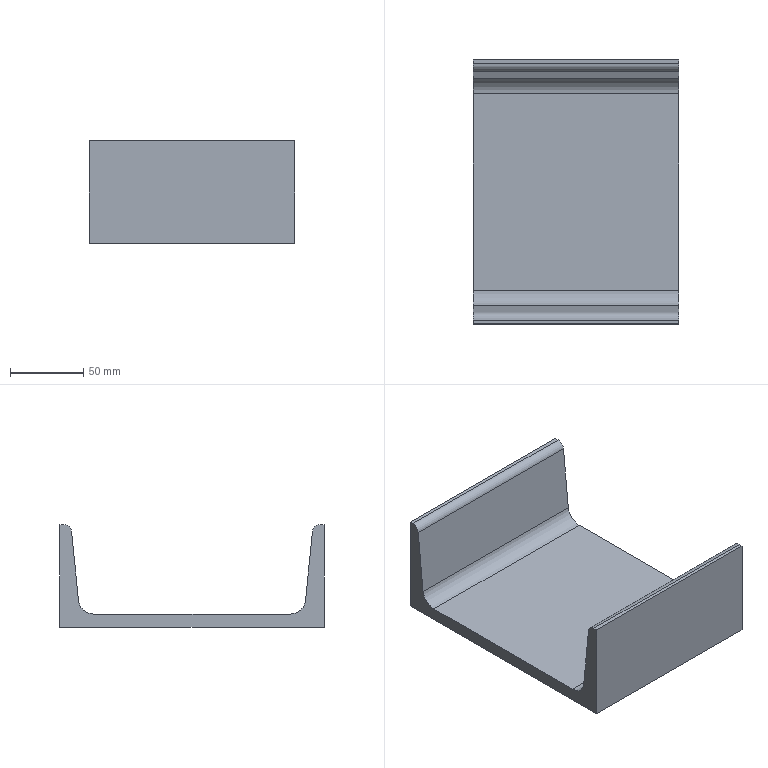Part | STEP file | 18# B Channel 140 (GB_INTERCHANGEABLE_PARTS_TM_SS 18X140)_GB_INTERCHANGEABLE_PARTS_TM_SS 18X140 | 1 solid | 14 faces | box 140 x 180 x 70 mm | volume 410063 mm3 | plane 10 | cylinder 4 | commonest cylinder face diameters 10.5 x2 21 x2
STEP:
#1=CARTESIAN_POINT('',(0.,0.,0.));
#2=DIRECTION('',(0.,0.,1.));
#3=DIRECTION('',(1.,0.,0.));
#4=AXIS2_PLACEMENT_3D('',#1,#2,#3);
#5=CARTESIAN_POINT('',(140.,82.077,65.272));
#6=VERTEX_POINT('',#5);
#7=CARTESIAN_POINT('',(140.,77.396,18.455));
#8=VERTEX_POINT('',#7);
#9=CARTESIAN_POINT('',(140.,76.45,9.));
#10=DIRECTION('',(0.,-0.0995,-0.995));
#11=VECTOR('',#10,1.);
#12=LINE('',#9,#11);
#13=CARTESIAN_POINT('',(140.,76.45,9.));
#14=DIRECTION('',(0.,0.995,-0.0995));
#15=DIRECTION('',(0.,0.0995,0.995));
#16=AXIS2_PLACEMENT_3D('',#13,#14,#15);
#17=PLANE('',#16);
#18=CARTESIAN_POINT('',(0.,0.));
#19=DIRECTION('',(-1.,0.));
#20=VECTOR('',#19,1.);
#21=LINE('',#18,#20);
#22=(GEOMETRIC_REPRESENTATION_CONTEXT(2)PARAMETRIC_REPRESENTATION_CONTEXT()REPRESENTATION_CONTEXT('',''));
#23=DEFINITIONAL_REPRESENTATION('',(#21),#22);
#24=PCURVE('',#17,#23);
#25=CARTESIAN_POINT('',(140.,75.55,0.));
#26=DIRECTION('',(1.,0.,0.));
#27=DIRECTION('',(0.,0.,-1.));
#28=AXIS2_PLACEMENT_3D('',#25,#26,#27);
#29=PLANE('',#28);
#30=CARTESIAN_POINT('',(-9.,0.9));
#31=DIRECTION('',(0.995,-0.0995));
#32=VECTOR('',#31,1.);
#33=LINE('',#30,#32);
#34=(GEOMETRIC_REPRESENTATION_CONTEXT(2)PARAMETRIC_REPRESENTATION_CONTEXT()REPRESENTATION_CONTEXT('',''));
#35=DEFINITIONAL_REPRESENTATION('',(#33),#34);
#36=PCURVE('',#29,#35);
#37=SURFACE_CURVE('',#12,(#24,#36),.PCURVE_S1.);
#38=EDGE_CURVE('',#6,#8,#37,.T.);
#39=ORIENTED_EDGE('',*,*,#38,.F.);
#40=CARTESIAN_POINT('',(0.,82.077,65.272));
#41=VERTEX_POINT('',#40);
#42=CARTESIAN_POINT('',(140.,82.077,65.272));
#43=DIRECTION('',(-1.,0.,0.));
#44=VECTOR('',#43,1.);
#45=LINE('',#42,#44);
#46=CARTESIAN_POINT('',(56.553,0.));
#47=DIRECTION('',(0.,-1.));
#48=VECTOR('',#47,1.);
#49=LINE('',#46,#48);
#50=(GEOMETRIC_REPRESENTATION_CONTEXT(2)PARAMETRIC_REPRESENTATION_CONTEXT()REPRESENTATION_CONTEXT('',''));
#51=DEFINITIONAL_REPRESENTATION('',(#49),#50);
#52=PCURVE('',#17,#51);
#53=CARTESIAN_POINT('',(140.,87.301,64.75));
#54=DIRECTION('',(-1.,0.,0.));
#55=DIRECTION('',(0.,0.,1.));
#56=AXIS2_PLACEMENT_3D('',#53,#54,#55);
#57=CYLINDRICAL_SURFACE('',#56,5.25);
#58=CARTESIAN_POINT('',(4.812,0.));
#59=DIRECTION('',(0.,1.));
#60=VECTOR('',#59,1.);
#61=LINE('',#58,#60);
#62=(GEOMETRIC_REPRESENTATION_CONTEXT(2)PARAMETRIC_REPRESENTATION_CONTEXT()REPRESENTATION_CONTEXT('',''));
#63=DEFINITIONAL_REPRESENTATION('',(#61),#62);
#64=PCURVE('',#57,#63);
#65=SURFACE_CURVE('',#45,(#52,#64),.PCURVE_S1.);
#66=EDGE_CURVE('',#6,#41,#65,.T.);
#67=ORIENTED_EDGE('',*,*,#66,.T.);
#68=CARTESIAN_POINT('',(0.,77.396,18.455));
#69=VERTEX_POINT('',#68);
#70=CARTESIAN_POINT('',(0.,76.45,9.));
#71=DIRECTION('',(0.,-0.0995,-0.995));
#72=VECTOR('',#71,1.);
#73=LINE('',#70,#72);
#74=CARTESIAN_POINT('',(0.,-140.));
#75=DIRECTION('',(-1.,0.));
#76=VECTOR('',#75,1.);
#77=LINE('',#74,#76);
#78=(GEOMETRIC_REPRESENTATION_CONTEXT(2)PARAMETRIC_REPRESENTATION_CONTEXT()REPRESENTATION_CONTEXT('',''));
#79=DEFINITIONAL_REPRESENTATION('',(#77),#78);
#80=PCURVE('',#17,#79);
#81=CARTESIAN_POINT('',(0.,75.55,0.));
#82=DIRECTION('',(1.,0.,0.));
#83=DIRECTION('',(0.,0.,-1.));
#84=AXIS2_PLACEMENT_3D('',#81,#82,#83);
#85=PLANE('',#84);
#86=CARTESIAN_POINT('',(-9.,0.9));
#87=DIRECTION('',(0.995,-0.0995));
#88=VECTOR('',#87,1.);
#89=LINE('',#86,#88);
#90=(GEOMETRIC_REPRESENTATION_CONTEXT(2)PARAMETRIC_REPRESENTATION_CONTEXT()REPRESENTATION_CONTEXT('',''));
#91=DEFINITIONAL_REPRESENTATION('',(#89),#90);
#92=PCURVE('',#85,#91);
#93=SURFACE_CURVE('',#73,(#80,#92),.PCURVE_S1.);
#94=EDGE_CURVE('',#41,#69,#93,.T.);
#95=ORIENTED_EDGE('',*,*,#94,.T.);
#96=CARTESIAN_POINT('',(140.,77.396,18.455));
#97=DIRECTION('',(1.,0.,0.));
#98=VECTOR('',#97,1.);
#99=LINE('',#96,#98);
#100=CARTESIAN_POINT('',(9.502,0.));
#101=DIRECTION('',(0.,1.));
#102=VECTOR('',#101,1.);
#103=LINE('',#100,#102);
#104=(GEOMETRIC_REPRESENTATION_CONTEXT(2)PARAMETRIC_REPRESENTATION_CONTEXT()REPRESENTATION_CONTEXT('',''));
#105=DEFINITIONAL_REPRESENTATION('',(#103),#104);
#106=PCURVE('',#17,#105);
#107=CARTESIAN_POINT('',(140.,66.948,19.5));
#108=DIRECTION('',(1.,0.,0.));
#109=DIRECTION('',(0.,0.,-1.));
#110=AXIS2_PLACEMENT_3D('',#107,#108,#109);
#111=CYLINDRICAL_SURFACE('',#110,10.5);
#112=CARTESIAN_POINT('',(1.471,0.));
#113=DIRECTION('',(0.,1.));
#114=VECTOR('',#113,1.);
#115=LINE('',#112,#114);
#116=(GEOMETRIC_REPRESENTATION_CONTEXT(2)PARAMETRIC_REPRESENTATION_CONTEXT()REPRESENTATION_CONTEXT('',''));
#117=DEFINITIONAL_REPRESENTATION('',(#115),#116);
#118=PCURVE('',#111,#117);
#119=SURFACE_CURVE('',#99,(#106,#118),.PCURVE_S1.);
#120=EDGE_CURVE('',#69,#8,#119,.T.);
#121=ORIENTED_EDGE('',*,*,#120,.T.);
#122=EDGE_LOOP('',(#39,#67,#95,#121));
#123=FACE_BOUND('',#122,.T.);
#124=ADVANCED_FACE('',(#123),#17,.F.);
#125=CARTESIAN_POINT('',(0.,66.948,9.));
#126=VERTEX_POINT('',#125);
#127=CARTESIAN_POINT('',(0.,-66.948,9.));
#128=VERTEX_POINT('',#127);
#129=CARTESIAN_POINT('',(0.,-76.45,9.));
#130=DIRECTION('',(0.,-1.,0.));
#131=VECTOR('',#130,1.);
#132=LINE('',#129,#131);
#133=CARTESIAN_POINT('',(140.,-76.45,9.));
#134=DIRECTION('',(0.,0.,-1.));
#135=DIRECTION('',(-1.,0.,0.));
#136=AXIS2_PLACEMENT_3D('',#133,#134,#135);
#137=PLANE('',#136);
#138=CARTESIAN_POINT('',(140.,0.));
#139=DIRECTION('',(0.,-1.));
#140=VECTOR('',#139,1.);
#141=LINE('',#138,#140);
#142=(GEOMETRIC_REPRESENTATION_CONTEXT(2)PARAMETRIC_REPRESENTATION_CONTEXT()REPRESENTATION_CONTEXT('',''));
#143=DEFINITIONAL_REPRESENTATION('',(#141),#142);
#144=PCURVE('',#137,#143);
#145=CARTESIAN_POINT('',(-9.,-152.));
#146=DIRECTION('',(0.,-1.));
#147=VECTOR('',#146,1.);
#148=LINE('',#145,#147);
#149=(GEOMETRIC_REPRESENTATION_CONTEXT(2)PARAMETRIC_REPRESENTATION_CONTEXT()REPRESENTATION_CONTEXT('',''));
#150=DEFINITIONAL_REPRESENTATION('',(#148),#149);
#151=PCURVE('',#85,#150);
#152=SURFACE_CURVE('',#132,(#144,#151),.PCURVE_S1.);
#153=EDGE_CURVE('',#126,#128,#152,.T.);
#154=ORIENTED_EDGE('',*,*,#153,.T.);
#155=CARTESIAN_POINT('',(140.,-66.948,9.));
#156=VERTEX_POINT('',#155);
#157=CARTESIAN_POINT('',(140.,-66.948,9.));
#158=DIRECTION('',(1.,0.,0.));
#159=VECTOR('',#158,1.);
#160=LINE('',#157,#159);
#161=CARTESIAN_POINT('',(0.,9.502));
#162=DIRECTION('',(-1.,0.));
#163=VECTOR('',#162,1.);
#164=LINE('',#161,#163);
#165=(GEOMETRIC_REPRESENTATION_CONTEXT(2)PARAMETRIC_REPRESENTATION_CONTEXT()REPRESENTATION_CONTEXT('',''));
#166=DEFINITIONAL_REPRESENTATION('',(#164),#165);
#167=PCURVE('',#137,#166);
#168=CARTESIAN_POINT('',(140.,-66.948,19.5));
#169=DIRECTION('',(1.,0.,0.));
#170=DIRECTION('',(0.,0.,-1.));
#171=AXIS2_PLACEMENT_3D('',#168,#169,#170);
#172=CYLINDRICAL_SURFACE('',#171,10.5);
#173=CARTESIAN_POINT('',(6.283,0.));
#174=DIRECTION('',(0.,1.));
#175=VECTOR('',#174,1.);
#176=LINE('',#173,#175);
#177=(GEOMETRIC_REPRESENTATION_CONTEXT(2)PARAMETRIC_REPRESENTATION_CONTEXT()REPRESENTATION_CONTEXT('',''));
#178=DEFINITIONAL_REPRESENTATION('',(#176),#177);
#179=PCURVE('',#172,#178);
#180=SURFACE_CURVE('',#160,(#167,#179),.PCURVE_S1.);
#181=EDGE_CURVE('',#128,#156,#180,.T.);
#182=ORIENTED_EDGE('',*,*,#181,.T.);
#183=CARTESIAN_POINT('',(140.,66.948,9.));
#184=VERTEX_POINT('',#183);
#185=CARTESIAN_POINT('',(140.,-76.45,9.));
#186=DIRECTION('',(0.,-1.,0.));
#187=VECTOR('',#186,1.);
#188=LINE('',#185,#187);
#189=CARTESIAN_POINT('',(0.,0.));
#190=DIRECTION('',(0.,-1.));
#191=VECTOR('',#190,1.);
#192=LINE('',#189,#191);
#193=(GEOMETRIC_REPRESENTATION_CONTEXT(2)PARAMETRIC_REPRESENTATION_CONTEXT()REPRESENTATION_CONTEXT('',''));
#194=DEFINITIONAL_REPRESENTATION('',(#192),#193);
#195=PCURVE('',#137,#194);
#196=CARTESIAN_POINT('',(-9.,-152.));
#197=DIRECTION('',(0.,-1.));
#198=VECTOR('',#197,1.);
#199=LINE('',#196,#198);
#200=(GEOMETRIC_REPRESENTATION_CONTEXT(2)PARAMETRIC_REPRESENTATION_CONTEXT()REPRESENTATION_CONTEXT('',''));
#201=DEFINITIONAL_REPRESENTATION('',(#199),#200);
#202=PCURVE('',#29,#201);
#203=SURFACE_CURVE('',#188,(#195,#202),.PCURVE_S1.);
#204=EDGE_CURVE('',#184,#156,#203,.T.);
#205=ORIENTED_EDGE('',*,*,#204,.F.);
#206=CARTESIAN_POINT('',(0.,66.948,9.));
#207=DIRECTION('',(-1.,0.,0.));
#208=VECTOR('',#207,1.);
#209=LINE('',#206,#208);
#210=CARTESIAN_POINT('',(140.,143.398));
#211=DIRECTION('',(1.,0.));
#212=VECTOR('',#211,1.);
#213=LINE('',#210,#212);
#214=(GEOMETRIC_REPRESENTATION_CONTEXT(2)PARAMETRIC_REPRESENTATION_CONTEXT()REPRESENTATION_CONTEXT('',''));
#215=DEFINITIONAL_REPRESENTATION('',(#213),#214);
#216=PCURVE('',#137,#215);
#217=CARTESIAN_POINT('',(0.,-140.));
#218=DIRECTION('',(0.,-1.));
#219=VECTOR('',#218,1.);
#220=LINE('',#217,#219);
#221=(GEOMETRIC_REPRESENTATION_CONTEXT(2)PARAMETRIC_REPRESENTATION_CONTEXT()REPRESENTATION_CONTEXT('',''));
#222=DEFINITIONAL_REPRESENTATION('',(#220),#221);
#223=PCURVE('',#111,#222);
#224=SURFACE_CURVE('',#209,(#216,#223),.PCURVE_S1.);
#225=EDGE_CURVE('',#184,#126,#224,.T.);
#226=ORIENTED_EDGE('',*,*,#225,.T.);
#227=EDGE_LOOP('',(#154,#182,#205,#226));
#228=FACE_BOUND('',#227,.T.);
#229=ADVANCED_FACE('',(#228),#137,.F.);
#230=CARTESIAN_POINT('',(0.,-77.396,18.455));
#231=VERTEX_POINT('',#230);
#232=CARTESIAN_POINT('',(0.,-82.077,65.272));
#233=VERTEX_POINT('',#232);
#234=CARTESIAN_POINT('',(0.,-76.45,9.));
#235=DIRECTION('',(0.,-0.0995,0.995));
#236=VECTOR('',#235,1.);
#237=LINE('',#234,#236);
#238=CARTESIAN_POINT('',(140.,-76.45,9.));
#239=DIRECTION('',(0.,-0.995,-0.0995));
#240=DIRECTION('',(0.,0.0995,-0.995));
#241=AXIS2_PLACEMENT_3D('',#238,#239,#240);
#242=PLANE('',#241);
#243=CARTESIAN_POINT('',(0.,-140.));
#244=DIRECTION('',(-1.,0.));
#245=VECTOR('',#244,1.);
#246=LINE('',#243,#245);
#247=(GEOMETRIC_REPRESENTATION_CONTEXT(2)PARAMETRIC_REPRESENTATION_CONTEXT()REPRESENTATION_CONTEXT('',''));
#248=DEFINITIONAL_REPRESENTATION('',(#246),#247);
#249=PCURVE('',#242,#248);
#250=CARTESIAN_POINT('',(-9.,-152.));
#251=DIRECTION('',(-0.995,-0.0995));
#252=VECTOR('',#251,1.);
#253=LINE('',#250,#252);
#254=(GEOMETRIC_REPRESENTATION_CONTEXT(2)PARAMETRIC_REPRESENTATION_CONTEXT()REPRESENTATION_CONTEXT('',''));
#255=DEFINITIONAL_REPRESENTATION('',(#253),#254);
#256=PCURVE('',#85,#255);
#257=SURFACE_CURVE('',#237,(#249,#256),.PCURVE_S1.);
#258=EDGE_CURVE('',#231,#233,#257,.T.);
#259=ORIENTED_EDGE('',*,*,#258,.T.);
#260=CARTESIAN_POINT('',(140.,-82.077,65.272));
#261=VERTEX_POINT('',#260);
#262=CARTESIAN_POINT('',(140.,-82.077,65.272));
#263=DIRECTION('',(1.,0.,0.));
#264=VECTOR('',#263,1.);
#265=LINE('',#262,#264);
#266=CARTESIAN_POINT('',(-56.553,0.));
#267=DIRECTION('',(0.,1.));
#268=VECTOR('',#267,1.);
#269=LINE('',#266,#268);
#270=(GEOMETRIC_REPRESENTATION_CONTEXT(2)PARAMETRIC_REPRESENTATION_CONTEXT()REPRESENTATION_CONTEXT('',''));
#271=DEFINITIONAL_REPRESENTATION('',(#269),#270);
#272=PCURVE('',#242,#271);
#273=CARTESIAN_POINT('',(140.,-87.301,64.75));
#274=DIRECTION('',(-1.,0.,0.));
#275=DIRECTION('',(0.,0.,1.));
#276=AXIS2_PLACEMENT_3D('',#273,#274,#275);
#277=CYLINDRICAL_SURFACE('',#276,5.25);
#278=CARTESIAN_POINT('',(1.471,0.));
#279=DIRECTION('',(0.,-1.));
#280=VECTOR('',#279,1.);
#281=LINE('',#278,#280);
#282=(GEOMETRIC_REPRESENTATION_CONTEXT(2)PARAMETRIC_REPRESENTATION_CONTEXT()REPRESENTATION_CONTEXT('',''));
#283=DEFINITIONAL_REPRESENTATION('',(#281),#282);
#284=PCURVE('',#277,#283);
#285=SURFACE_CURVE('',#265,(#272,#284),.PCURVE_S1.);
#286=EDGE_CURVE('',#233,#261,#285,.T.);
#287=ORIENTED_EDGE('',*,*,#286,.T.);
#288=CARTESIAN_POINT('',(140.,-77.396,18.455));
#289=VERTEX_POINT('',#288);
#290=CARTESIAN_POINT('',(140.,-76.45,9.));
#291=DIRECTION('',(0.,-0.0995,0.995));
#292=VECTOR('',#291,1.);
#293=LINE('',#290,#292);
#294=CARTESIAN_POINT('',(0.,0.));
#295=DIRECTION('',(-1.,0.));
#296=VECTOR('',#295,1.);
#297=LINE('',#294,#296);
#298=(GEOMETRIC_REPRESENTATION_CONTEXT(2)PARAMETRIC_REPRESENTATION_CONTEXT()REPRESENTATION_CONTEXT('',''));
#299=DEFINITIONAL_REPRESENTATION('',(#297),#298);
#300=PCURVE('',#242,#299);
#301=CARTESIAN_POINT('',(-9.,-152.));
#302=DIRECTION('',(-0.995,-0.0995));
#303=VECTOR('',#302,1.);
#304=LINE('',#301,#303);
#305=(GEOMETRIC_REPRESENTATION_CONTEXT(2)PARAMETRIC_REPRESENTATION_CONTEXT()REPRESENTATION_CONTEXT('',''));
#306=DEFINITIONAL_REPRESENTATION('',(#304),#305);
#307=PCURVE('',#29,#306);
#308=SURFACE_CURVE('',#293,(#300,#307),.PCURVE_S1.);
#309=EDGE_CURVE('',#289,#261,#308,.T.);
#310=ORIENTED_EDGE('',*,*,#309,.F.);
#311=CARTESIAN_POINT('',(0.,-77.396,18.455));
#312=DIRECTION('',(-1.,0.,0.));
#313=VECTOR('',#312,1.);
#314=LINE('',#311,#313);
#315=CARTESIAN_POINT('',(-9.502,-140.));
#316=DIRECTION('',(0.,-1.));
#317=VECTOR('',#316,1.);
#318=LINE('',#315,#317);
#319=(GEOMETRIC_REPRESENTATION_CONTEXT(2)PARAMETRIC_REPRESENTATION_CONTEXT()REPRESENTATION_CONTEXT('',''));
#320=DEFINITIONAL_REPRESENTATION('',(#318),#319);
#321=PCURVE('',#242,#320);
#322=CARTESIAN_POINT('',(4.812,-140.));
#323=DIRECTION('',(0.,-1.));
#324=VECTOR('',#323,1.);
#325=LINE('',#322,#324);
#326=(GEOMETRIC_REPRESENTATION_CONTEXT(2)PARAMETRIC_REPRESENTATION_CONTEXT()REPRESENTATION_CONTEXT('',''));
#327=DEFINITIONAL_REPRESENTATION('',(#325),#326);
#328=PCURVE('',#172,#327);
#329=SURFACE_CURVE('',#314,(#321,#328),.PCURVE_S1.);
#330=EDGE_CURVE('',#289,#231,#329,.T.);
#331=ORIENTED_EDGE('',*,*,#330,.T.);
#332=EDGE_LOOP('',(#259,#287,#310,#331));
#333=FACE_BOUND('',#332,.T.);
#334=ADVANCED_FACE('',(#333),#242,.F.);
#335=CARTESIAN_POINT('',(140.,-87.301,70.));
#336=VERTEX_POINT('',#335);
#337=CARTESIAN_POINT('',(140.,-90.,70.));
#338=VERTEX_POINT('',#337);
#339=CARTESIAN_POINT('',(140.,-82.55,70.));
#340=DIRECTION('',(0.,-1.,0.));
#341=VECTOR('',#340,1.);
#342=LINE('',#339,#341);
#343=CARTESIAN_POINT('',(140.,-82.55,70.));
#344=DIRECTION('',(0.,0.,-1.));
#345=DIRECTION('',(-1.,0.,0.));
#346=AXIS2_PLACEMENT_3D('',#343,#344,#345);
#347=PLANE('',#346);
#348=CARTESIAN_POINT('',(0.,0.));
#349=DIRECTION('',(0.,-1.));
#350=VECTOR('',#349,1.);
#351=LINE('',#348,#350);
#352=(GEOMETRIC_REPRESENTATION_CONTEXT(2)PARAMETRIC_REPRESENTATION_CONTEXT()REPRESENTATION_CONTEXT('',''));
#353=DEFINITIONAL_REPRESENTATION('',(#351),#352);
#354=PCURVE('',#347,#353);
#355=CARTESIAN_POINT('',(-70.,-158.1));
#356=DIRECTION('',(0.,-1.));
#357=VECTOR('',#356,1.);
#358=LINE('',#355,#357);
#359=(GEOMETRIC_REPRESENTATION_CONTEXT(2)PARAMETRIC_REPRESENTATION_CONTEXT()REPRESENTATION_CONTEXT('',''));
#360=DEFINITIONAL_REPRESENTATION('',(#358),#359);
#361=PCURVE('',#29,#360);
#362=SURFACE_CURVE('',#342,(#354,#361),.PCURVE_S1.);
#363=EDGE_CURVE('',#336,#338,#362,.T.);
#364=ORIENTED_EDGE('',*,*,#363,.F.);
#365=CARTESIAN_POINT('',(0.,-87.301,70.));
#366=VERTEX_POINT('',#365);
#367=CARTESIAN_POINT('',(140.,-87.301,70.));
#368=DIRECTION('',(-1.,0.,0.));
#369=VECTOR('',#368,1.);
#370=LINE('',#367,#369);
#371=CARTESIAN_POINT('',(0.,-4.751));
#372=DIRECTION('',(1.,0.));
#373=VECTOR('',#372,1.);
#374=LINE('',#371,#373);
#375=(GEOMETRIC_REPRESENTATION_CONTEXT(2)PARAMETRIC_REPRESENTATION_CONTEXT()REPRESENTATION_CONTEXT('',''));
#376=DEFINITIONAL_REPRESENTATION('',(#374),#375);
#377=PCURVE('',#347,#376);
#378=CARTESIAN_POINT('',(0.,0.));
#379=DIRECTION('',(0.,1.));
#380=VECTOR('',#379,1.);
#381=LINE('',#378,#380);
#382=(GEOMETRIC_REPRESENTATION_CONTEXT(2)PARAMETRIC_REPRESENTATION_CONTEXT()REPRESENTATION_CONTEXT('',''));
#383=DEFINITIONAL_REPRESENTATION('',(#381),#382);
#384=PCURVE('',#277,#383);
#385=SURFACE_CURVE('',#370,(#377,#384),.PCURVE_S1.);
#386=EDGE_CURVE('',#336,#366,#385,.T.);
#387=ORIENTED_EDGE('',*,*,#386,.T.);
#388=CARTESIAN_POINT('',(0.,-90.,70.));
#389=VERTEX_POINT('',#388);
#390=CARTESIAN_POINT('',(0.,-82.55,70.));
#391=DIRECTION('',(0.,-1.,0.));
#392=VECTOR('',#391,1.);
#393=LINE('',#390,#392);
#394=CARTESIAN_POINT('',(140.,0.));
#395=DIRECTION('',(0.,-1.));
#396=VECTOR('',#395,1.);
#397=LINE('',#394,#396);
#398=(GEOMETRIC_REPRESENTATION_CONTEXT(2)PARAMETRIC_REPRESENTATION_CONTEXT()REPRESENTATION_CONTEXT('',''));
#399=DEFINITIONAL_REPRESENTATION('',(#397),#398);
#400=PCURVE('',#347,#399);
#401=CARTESIAN_POINT('',(-70.,-158.1));
#402=DIRECTION('',(0.,-1.));
#403=VECTOR('',#402,1.);
#404=LINE('',#401,#403);
#405=(GEOMETRIC_REPRESENTATION_CONTEXT(2)PARAMETRIC_REPRESENTATION_CONTEXT()REPRESENTATION_CONTEXT('',''));
#406=DEFINITIONAL_REPRESENTATION('',(#404),#405);
#407=PCURVE('',#85,#406);
#408=SURFACE_CURVE('',#393,(#400,#407),.PCURVE_S1.);
#409=EDGE_CURVE('',#366,#389,#408,.T.);
#410=ORIENTED_EDGE('',*,*,#409,.T.);
#411=CARTESIAN_POINT('',(140.,-90.,70.));
#412=DIRECTION('',(-1.,0.,0.));
#413=VECTOR('',#412,1.);
#414=LINE('',#411,#413);
#415=CARTESIAN_POINT('',(0.,-7.45));
#416=DIRECTION('',(1.,0.));
#417=VECTOR('',#416,1.);
#418=LINE('',#415,#417);
#419=(GEOMETRIC_REPRESENTATION_CONTEXT(2)PARAMETRIC_REPRESENTATION_CONTEXT()REPRESENTATION_CONTEXT('',''));
#420=DEFINITIONAL_REPRESENTATION('',(#418),#419);
#421=PCURVE('',#347,#420);
#422=CARTESIAN_POINT('',(140.,-90.,0.));
#423=DIRECTION('',(0.,1.,0.));
#424=DIRECTION('',(0.,0.,1.));
#425=AXIS2_PLACEMENT_3D('',#422,#423,#424);
#426=PLANE('',#425);
#427=CARTESIAN_POINT('',(70.,0.));
#428=DIRECTION('',(0.,-1.));
#429=VECTOR('',#428,1.);
#430=LINE('',#427,#429);
#431=(GEOMETRIC_REPRESENTATION_CONTEXT(2)PARAMETRIC_REPRESENTATION_CONTEXT()REPRESENTATION_CONTEXT('',''));
#432=DEFINITIONAL_REPRESENTATION('',(#430),#431);
#433=PCURVE('',#426,#432);
#434=SURFACE_CURVE('',#414,(#421,#433),.PCURVE_S1.);
#435=EDGE_CURVE('',#338,#389,#434,.T.);
#436=ORIENTED_EDGE('',*,*,#435,.F.);
#437=EDGE_LOOP('',(#364,#387,#410,#436));
#438=FACE_BOUND('',#437,.T.);
#439=ADVANCED_FACE('',(#438),#347,.F.);
#440=CARTESIAN_POINT('',(0.,-90.,0.));
#441=VERTEX_POINT('',#440);
#442=CARTESIAN_POINT('',(0.,-90.,0.));
#443=DIRECTION('',(0.,0.,-1.));
#444=VECTOR('',#443,1.);
#445=LINE('',#442,#444);
#446=CARTESIAN_POINT('',(0.,-140.));
#447=DIRECTION('',(-1.,0.));
#448=VECTOR('',#447,1.);
#449=LINE('',#446,#448);
#450=(GEOMETRIC_REPRESENTATION_CONTEXT(2)PARAMETRIC_REPRESENTATION_CONTEXT()REPRESENTATION_CONTEXT('',''));
#451=DEFINITIONAL_REPRESENTATION('',(#449),#450);
#452=PCURVE('',#426,#451);
#453=CARTESIAN_POINT('',(0.,-165.55));
#454=DIRECTION('',(1.,0.));
#455=VECTOR('',#454,1.);
#456=LINE('',#453,#455);
#457=(GEOMETRIC_REPRESENTATION_CONTEXT(2)PARAMETRIC_REPRESENTATION_CONTEXT()REPRESENTATION_CONTEXT('',''));
#458=DEFINITIONAL_REPRESENTATION('',(#456),#457);
#459=PCURVE('',#85,#458);
#460=SURFACE_CURVE('',#445,(#452,#459),.PCURVE_S1.);
#461=EDGE_CURVE('',#389,#441,#460,.T.);
#462=ORIENTED_EDGE('',*,*,#461,.T.);
#463=CARTESIAN_POINT('',(140.,-90.,0.));
#464=VERTEX_POINT('',#463);
#465=CARTESIAN_POINT('',(140.,-90.,0.));
#466=DIRECTION('',(-1.,0.,0.));
#467=VECTOR('',#466,1.);
#468=LINE('',#465,#467);
#469=CARTESIAN_POINT('',(0.,0.));
#470=DIRECTION('',(0.,-1.));
#471=VECTOR('',#470,1.);
#472=LINE('',#469,#471);
#473=(GEOMETRIC_REPRESENTATION_CONTEXT(2)PARAMETRIC_REPRESENTATION_CONTEXT()REPRESENTATION_CONTEXT('',''));
#474=DEFINITIONAL_REPRESENTATION('',(#472),#473);
#475=PCURVE('',#426,#474);
#476=CARTESIAN_POINT('',(140.,90.,0.));
#477=DIRECTION('',(0.,0.,1.));
#478=DIRECTION('',(0.,-1.,0.));
#479=AXIS2_PLACEMENT_3D('',#476,#477,#478);
#480=PLANE('',#479);
#481=CARTESIAN_POINT('',(180.,0.));
#482=DIRECTION('',(0.,-1.));
#483=VECTOR('',#482,1.);
#484=LINE('',#481,#483);
#485=(GEOMETRIC_REPRESENTATION_CONTEXT(2)PARAMETRIC_REPRESENTATION_CONTEXT()REPRESENTATION_CONTEXT('',''));
#486=DEFINITIONAL_REPRESENTATION('',(#484),#485);
#487=PCURVE('',#480,#486);
#488=SURFACE_CURVE('',#468,(#475,#487),.PCURVE_S1.);
#489=EDGE_CURVE('',#464,#441,#488,.T.);
#490=ORIENTED_EDGE('',*,*,#489,.F.);
#491=CARTESIAN_POINT('',(140.,-90.,0.));
#492=DIRECTION('',(0.,0.,-1.));
#493=VECTOR('',#492,1.);
#494=LINE('',#491,#493);
#495=CARTESIAN_POINT('',(0.,0.));
#496=DIRECTION('',(-1.,0.));
#497=VECTOR('',#496,1.);
#498=LINE('',#495,#497);
#499=(GEOMETRIC_REPRESENTATION_CONTEXT(2)PARAMETRIC_REPRESENTATION_CONTEXT()REPRESENTATION_CONTEXT('',''));
#500=DEFINITIONAL_REPRESENTATION('',(#498),#499);
#501=PCURVE('',#426,#500);
#502=CARTESIAN_POINT('',(0.,-165.55));
#503=DIRECTION('',(1.,0.));
#504=VECTOR('',#503,1.);
#505=LINE('',#502,#504);
#506=(GEOMETRIC_REPRESENTATION_CONTEXT(2)PARAMETRIC_REPRESENTATION_CONTEXT()REPRESENTATION_CONTEXT('',''));
#507=DEFINITIONAL_REPRESENTATION('',(#505),#506);
#508=PCURVE('',#29,#507);
#509=SURFACE_CURVE('',#494,(#501,#508),.PCURVE_S1.);
#510=EDGE_CURVE('',#338,#464,#509,.T.);
#511=ORIENTED_EDGE('',*,*,#510,.F.);
#512=ORIENTED_EDGE('',*,*,#435,.T.);
#513=EDGE_LOOP('',(#462,#490,#511,#512));
#514=FACE_BOUND('',#513,.T.);
#515=ADVANCED_FACE('',(#514),#426,.F.);
#516=CARTESIAN_POINT('',(0.,90.,0.));
#517=VERTEX_POINT('',#516);
#518=CARTESIAN_POINT('',(0.,90.,0.));
#519=DIRECTION('',(0.,1.,0.));
#520=VECTOR('',#519,1.);
#521=LINE('',#518,#520);
#522=CARTESIAN_POINT('',(0.,-140.));
#523=DIRECTION('',(-1.,0.));
#524=VECTOR('',#523,1.);
#525=LINE('',#522,#524);
#526=(GEOMETRIC_REPRESENTATION_CONTEXT(2)PARAMETRIC_REPRESENTATION_CONTEXT()REPRESENTATION_CONTEXT('',''));
#527=DEFINITIONAL_REPRESENTATION('',(#525),#526);
#528=PCURVE('',#480,#527);
#529=CARTESIAN_POINT('',(0.,14.45));
#530=DIRECTION('',(0.,1.));
#531=VECTOR('',#530,1.);
#532=LINE('',#529,#531);
#533=(GEOMETRIC_REPRESENTATION_CONTEXT(2)PARAMETRIC_REPRESENTATION_CONTEXT()REPRESENTATION_CONTEXT('',''));
#534=DEFINITIONAL_REPRESENTATION('',(#532),#533);
#535=PCURVE('',#85,#534);
#536=SURFACE_CURVE('',#521,(#528,#535),.PCURVE_S1.);
#537=EDGE_CURVE('',#441,#517,#536,.T.);
#538=ORIENTED_EDGE('',*,*,#537,.T.);
#539=CARTESIAN_POINT('',(140.,90.,0.));
#540=VERTEX_POINT('',#539);
#541=CARTESIAN_POINT('',(140.,90.,0.));
#542=DIRECTION('',(-1.,0.,0.));
#543=VECTOR('',#542,1.);
#544=LINE('',#541,#543);
#545=CARTESIAN_POINT('',(0.,0.));
#546=DIRECTION('',(0.,-1.));
#547=VECTOR('',#546,1.);
#548=LINE('',#545,#547);
#549=(GEOMETRIC_REPRESENTATION_CONTEXT(2)PARAMETRIC_REPRESENTATION_CONTEXT()REPRESENTATION_CONTEXT('',''));
#550=DEFINITIONAL_REPRESENTATION('',(#548),#549);
#551=PCURVE('',#480,#550);
#552=CARTESIAN_POINT('',(140.,90.,0.));
#553=DIRECTION('',(0.,-1.,0.));
#554=DIRECTION('',(0.,0.,-1.));
#555=AXIS2_PLACEMENT_3D('',#552,#553,#554);
#556=PLANE('',#555);
#557=CARTESIAN_POINT('',(0.,0.));
#558=DIRECTION('',(0.,-1.));
#559=VECTOR('',#558,1.);
#560=LINE('',#557,#559);
#561=(GEOMETRIC_REPRESENTATION_CONTEXT(2)PARAMETRIC_REPRESENTATION_CONTEXT()REPRESENTATION_CONTEXT('',''));
#562=DEFINITIONAL_REPRESENTATION('',(#560),#561);
#563=PCURVE('',#556,#562);
#564=SURFACE_CURVE('',#544,(#551,#563),.PCURVE_S1.);
#565=EDGE_CURVE('',#540,#517,#564,.T.);
#566=ORIENTED_EDGE('',*,*,#565,.F.);
#567=CARTESIAN_POINT('',(140.,90.,0.));
#568=DIRECTION('',(0.,1.,0.));
#569=VECTOR('',#568,1.);
#570=LINE('',#567,#569);
#571=CARTESIAN_POINT('',(0.,0.));
#572=DIRECTION('',(-1.,0.));
#573=VECTOR('',#572,1.);
#574=LINE('',#571,#573);
#575=(GEOMETRIC_REPRESENTATION_CONTEXT(2)PARAMETRIC_REPRESENTATION_CONTEXT()REPRESENTATION_CONTEXT('',''));
#576=DEFINITIONAL_REPRESENTATION('',(#574),#575);
#577=PCURVE('',#480,#576);
#578=CARTESIAN_POINT('',(0.,14.45));
#579=DIRECTION('',(0.,1.));
#580=VECTOR('',#579,1.);
#581=LINE('',#578,#580);
#582=(GEOMETRIC_REPRESENTATION_CONTEXT(2)PARAMETRIC_REPRESENTATION_CONTEXT()REPRESENTATION_CONTEXT('',''));
#583=DEFINITIONAL_REPRESENTATION('',(#581),#582);
#584=PCURVE('',#29,#583);
#585=SURFACE_CURVE('',#570,(#577,#584),.PCURVE_S1.);
#586=EDGE_CURVE('',#464,#540,#585,.T.);
#587=ORIENTED_EDGE('',*,*,#586,.F.);
#588=ORIENTED_EDGE('',*,*,#489,.T.);
#589=EDGE_LOOP('',(#538,#566,#587,#588));
#590=FACE_BOUND('',#589,.T.);
#591=ADVANCED_FACE('',(#590),#480,.F.);
#592=CARTESIAN_POINT('',(0.,90.,70.));
#593=VERTEX_POINT('',#592);
#594=CARTESIAN_POINT('',(0.,90.,0.));
#595=DIRECTION('',(0.,0.,1.));
#596=VECTOR('',#595,1.);
#597=LINE('',#594,#596);
#598=CARTESIAN_POINT('',(0.,-140.));
#599=DIRECTION('',(-1.,0.));
#600=VECTOR('',#599,1.);
#601=LINE('',#598,#600);
#602=(GEOMETRIC_REPRESENTATION_CONTEXT(2)PARAMETRIC_REPRESENTATION_CONTEXT()REPRESENTATION_CONTEXT('',''));
#603=DEFINITIONAL_REPRESENTATION('',(#601),#602);
#604=PCURVE('',#556,#603);
#605=CARTESIAN_POINT('',(0.,14.45));
#606=DIRECTION('',(-1.,0.));
#607=VECTOR('',#606,1.);
#608=LINE('',#605,#607);
#609=(GEOMETRIC_REPRESENTATION_CONTEXT(2)PARAMETRIC_REPRESENTATION_CONTEXT()REPRESENTATION_CONTEXT('',''));
#610=DEFINITIONAL_REPRESENTATION('',(#608),#609);
#611=PCURVE('',#85,#610);
#612=SURFACE_CURVE('',#597,(#604,#611),.PCURVE_S1.);
#613=EDGE_CURVE('',#517,#593,#612,.T.);
#614=ORIENTED_EDGE('',*,*,#613,.T.);
#615=CARTESIAN_POINT('',(140.,90.,70.));
#616=VERTEX_POINT('',#615);
#617=CARTESIAN_POINT('',(140.,90.,70.));
#618=DIRECTION('',(-1.,0.,0.));
#619=VECTOR('',#618,1.);
#620=LINE('',#617,#619);
#621=CARTESIAN_POINT('',(-70.,0.));
#622=DIRECTION('',(0.,-1.));
#623=VECTOR('',#622,1.);
#624=LINE('',#621,#623);
#625=(GEOMETRIC_REPRESENTATION_CONTEXT(2)PARAMETRIC_REPRESENTATION_CONTEXT()REPRESENTATION_CONTEXT('',''));
#626=DEFINITIONAL_REPRESENTATION('',(#624),#625);
#627=PCURVE('',#556,#626);
#628=CARTESIAN_POINT('',(140.,82.55,70.));
#629=DIRECTION('',(0.,0.,-1.));
#630=DIRECTION('',(-1.,0.,0.));
#631=AXIS2_PLACEMENT_3D('',#628,#629,#630);
#632=PLANE('',#631);
#633=CARTESIAN_POINT('',(0.,7.45));
#634=DIRECTION('',(1.,0.));
#635=VECTOR('',#634,1.);
#636=LINE('',#633,#635);
#637=(GEOMETRIC_REPRESENTATION_CONTEXT(2)PARAMETRIC_REPRESENTATION_CONTEXT()REPRESENTATION_CONTEXT('',''));
#638=DEFINITIONAL_REPRESENTATION('',(#636),#637);
#639=PCURVE('',#632,#638);
#640=SURFACE_CURVE('',#620,(#627,#639),.PCURVE_S1.);
#641=EDGE_CURVE('',#616,#593,#640,.T.);
#642=ORIENTED_EDGE('',*,*,#641,.F.);
#643=CARTESIAN_POINT('',(140.,90.,0.));
#644=DIRECTION('',(0.,0.,1.));
#645=VECTOR('',#644,1.);
#646=LINE('',#643,#645);
#647=CARTESIAN_POINT('',(0.,0.));
#648=DIRECTION('',(-1.,0.));
#649=VECTOR('',#648,1.);
#650=LINE('',#647,#649);
#651=(GEOMETRIC_REPRESENTATION_CONTEXT(2)PARAMETRIC_REPRESENTATION_CONTEXT()REPRESENTATION_CONTEXT('',''));
#652=DEFINITIONAL_REPRESENTATION('',(#650),#651);
#653=PCURVE('',#556,#652);
#654=CARTESIAN_POINT('',(0.,14.45));
#655=DIRECTION('',(-1.,0.));
#656=VECTOR('',#655,1.);
#657=LINE('',#654,#656);
#658=(GEOMETRIC_REPRESENTATION_CONTEXT(2)PARAMETRIC_REPRESENTATION_CONTEXT()REPRESENTATION_CONTEXT('',''));
#659=DEFINITIONAL_REPRESENTATION('',(#657),#658);
#660=PCURVE('',#29,#659);
#661=SURFACE_CURVE('',#646,(#653,#660),.PCURVE_S1.);
#662=EDGE_CURVE('',#540,#616,#661,.T.);
#663=ORIENTED_EDGE('',*,*,#662,.F.);
#664=ORIENTED_EDGE('',*,*,#565,.T.);
#665=EDGE_LOOP('',(#614,#642,#663,#664));
#666=FACE_BOUND('',#665,.T.);
#667=ADVANCED_FACE('',(#666),#556,.F.);
#668=CARTESIAN_POINT('',(0.,87.301,70.));
#669=VERTEX_POINT('',#668);
#670=CARTESIAN_POINT('',(0.,82.55,70.));
#671=DIRECTION('',(0.,-1.,0.));
#672=VECTOR('',#671,1.);
#673=LINE('',#670,#672);
#674=CARTESIAN_POINT('',(140.,0.));
#675=DIRECTION('',(0.,-1.));
#676=VECTOR('',#675,1.);
#677=LINE('',#674,#676);
#678=(GEOMETRIC_REPRESENTATION_CONTEXT(2)PARAMETRIC_REPRESENTATION_CONTEXT()REPRESENTATION_CONTEXT('',''));
#679=DEFINITIONAL_REPRESENTATION('',(#677),#678);
#680=PCURVE('',#632,#679);
#681=CARTESIAN_POINT('',(-70.,7.));
#682=DIRECTION('',(0.,-1.));
#683=VECTOR('',#682,1.);
#684=LINE('',#681,#683);
#685=(GEOMETRIC_REPRESENTATION_CONTEXT(2)PARAMETRIC_REPRESENTATION_CONTEXT()REPRESENTATION_CONTEXT('',''));
#686=DEFINITIONAL_REPRESENTATION('',(#684),#685);
#687=PCURVE('',#85,#686);
#688=SURFACE_CURVE('',#673,(#680,#687),.PCURVE_S1.);
#689=EDGE_CURVE('',#593,#669,#688,.T.);
#690=ORIENTED_EDGE('',*,*,#689,.T.);
#691=CARTESIAN_POINT('',(140.,87.301,70.));
#692=VERTEX_POINT('',#691);
#693=CARTESIAN_POINT('',(140.,87.301,70.));
#694=DIRECTION('',(1.,0.,0.));
#695=VECTOR('',#694,1.);
#696=LINE('',#693,#695);
#697=CARTESIAN_POINT('',(0.,4.751));
#698=DIRECTION('',(-1.,0.));
#699=VECTOR('',#698,1.);
#700=LINE('',#697,#699);
#701=(GEOMETRIC_REPRESENTATION_CONTEXT(2)PARAMETRIC_REPRESENTATION_CONTEXT()REPRESENTATION_CONTEXT('',''));
#702=DEFINITIONAL_REPRESENTATION('',(#700),#701);
#703=PCURVE('',#632,#702);
#704=CARTESIAN_POINT('',(6.283,0.));
#705=DIRECTION('',(0.,-1.));
#706=VECTOR('',#705,1.);
#707=LINE('',#704,#706);
#708=(GEOMETRIC_REPRESENTATION_CONTEXT(2)PARAMETRIC_REPRESENTATION_CONTEXT()REPRESENTATION_CONTEXT('',''));
#709=DEFINITIONAL_REPRESENTATION('',(#707),#708);
#710=PCURVE('',#57,#709);
#711=SURFACE_CURVE('',#696,(#703,#710),.PCURVE_S1.);
#712=EDGE_CURVE('',#669,#692,#711,.T.);
#713=ORIENTED_EDGE('',*,*,#712,.T.);
#714=CARTESIAN_POINT('',(140.,82.55,70.));
#715=DIRECTION('',(0.,-1.,0.));
#716=VECTOR('',#715,1.);
#717=LINE('',#714,#716);
#718=CARTESIAN_POINT('',(0.,0.));
#719=DIRECTION('',(0.,-1.));
#720=VECTOR('',#719,1.);
#721=LINE('',#718,#720);
#722=(GEOMETRIC_REPRESENTATION_CONTEXT(2)PARAMETRIC_REPRESENTATION_CONTEXT()REPRESENTATION_CONTEXT('',''));
#723=DEFINITIONAL_REPRESENTATION('',(#721),#722);
#724=PCURVE('',#632,#723);
#725=CARTESIAN_POINT('',(-70.,7.));
#726=DIRECTION('',(0.,-1.));
#727=VECTOR('',#726,1.);
#728=LINE('',#725,#727);
#729=(GEOMETRIC_REPRESENTATION_CONTEXT(2)PARAMETRIC_REPRESENTATION_CONTEXT()REPRESENTATION_CONTEXT('',''));
#730=DEFINITIONAL_REPRESENTATION('',(#728),#729);
#731=PCURVE('',#29,#730);
#732=SURFACE_CURVE('',#717,(#724,#731),.PCURVE_S1.);
#733=EDGE_CURVE('',#616,#692,#732,.T.);
#734=ORIENTED_EDGE('',*,*,#733,.F.);
#735=ORIENTED_EDGE('',*,*,#641,.T.);
#736=EDGE_LOOP('',(#690,#713,#734,#735));
#737=FACE_BOUND('',#736,.T.);
#738=ADVANCED_FACE('',(#737),#632,.F.);
#739=ORIENTED_EDGE('',*,*,#309,.T.);
#740=CARTESIAN_POINT('',(140.,-87.301,64.75));
#741=DIRECTION('',(1.,0.,0.));
#742=DIRECTION('',(0.,0.,-1.));
#743=AXIS2_PLACEMENT_3D('',#740,#741,#742);
#744=CIRCLE('',#743,5.25);
#745=CARTESIAN_POINT('',(-64.75,-162.851));
#746=DIRECTION('',(1.,0.));
#747=AXIS2_PLACEMENT_2D('',#745,#746);
#748=CIRCLE('',#747,5.25);
#749=(GEOMETRIC_REPRESENTATION_CONTEXT(2)PARAMETRIC_REPRESENTATION_CONTEXT()REPRESENTATION_CONTEXT('',''));
#750=DEFINITIONAL_REPRESENTATION('',(#748),#749);
#751=PCURVE('',#29,#750);
#752=CARTESIAN_POINT('',(3.142,0.));
#753=DIRECTION('',(-1.,0.));
#754=VECTOR('',#753,1.);
#755=LINE('',#752,#754);
#756=(GEOMETRIC_REPRESENTATION_CONTEXT(2)PARAMETRIC_REPRESENTATION_CONTEXT()REPRESENTATION_CONTEXT('',''));
#757=DEFINITIONAL_REPRESENTATION('',(#755),#756);
#758=PCURVE('',#277,#757);
#759=SURFACE_CURVE('',#744,(#751,#758),.PCURVE_S1.);
#760=EDGE_CURVE('',#261,#336,#759,.T.);
#761=ORIENTED_EDGE('',*,*,#760,.T.);
#762=ORIENTED_EDGE('',*,*,#363,.T.);
#763=ORIENTED_EDGE('',*,*,#510,.T.);
#764=ORIENTED_EDGE('',*,*,#586,.T.);
#765=ORIENTED_EDGE('',*,*,#662,.T.);
#766=ORIENTED_EDGE('',*,*,#733,.T.);
#767=CARTESIAN_POINT('',(140.,87.301,64.75));
#768=DIRECTION('',(1.,0.,0.));
#769=DIRECTION('',(0.,0.,-1.));
#770=AXIS2_PLACEMENT_3D('',#767,#768,#769);
#771=CIRCLE('',#770,5.25);
#772=CARTESIAN_POINT('',(-64.75,11.751));
#773=DIRECTION('',(1.,0.));
#774=AXIS2_PLACEMENT_2D('',#772,#773);
#775=CIRCLE('',#774,5.25);
#776=(GEOMETRIC_REPRESENTATION_CONTEXT(2)PARAMETRIC_REPRESENTATION_CONTEXT()REPRESENTATION_CONTEXT('',''));
#777=DEFINITIONAL_REPRESENTATION('',(#775),#776);
#778=PCURVE('',#29,#777);
#779=CARTESIAN_POINT('',(9.425,0.));
#780=DIRECTION('',(-1.,0.));
#781=VECTOR('',#780,1.);
#782=LINE('',#779,#781);
#783=(GEOMETRIC_REPRESENTATION_CONTEXT(2)PARAMETRIC_REPRESENTATION_CONTEXT()REPRESENTATION_CONTEXT('',''));
#784=DEFINITIONAL_REPRESENTATION('',(#782),#783);
#785=PCURVE('',#57,#784);
#786=SURFACE_CURVE('',#771,(#778,#785),.PCURVE_S1.);
#787=EDGE_CURVE('',#692,#6,#786,.T.);
#788=ORIENTED_EDGE('',*,*,#787,.T.);
#789=ORIENTED_EDGE('',*,*,#38,.T.);
#790=CARTESIAN_POINT('',(140.,66.948,19.5));
#791=DIRECTION('',(-1.,0.,0.));
#792=DIRECTION('',(0.,0.,-1.));
#793=AXIS2_PLACEMENT_3D('',#790,#791,#792);
#794=CIRCLE('',#793,10.5);
#795=CARTESIAN_POINT('',(-9.,-8.602));
#796=CARTESIAN_POINT('',(-9.,-26.789));
#797=CARTESIAN_POINT('',(-24.75,-17.696));
#798=CARTESIAN_POINT('',(-40.5,-8.602));
#799=CARTESIAN_POINT('',(-24.75,0.4909));
#800=CARTESIAN_POINT('',(-9.,9.584));
#801=CARTESIAN_POINT('',(-9.,-8.602));
#802=(BOUNDED_CURVE()B_SPLINE_CURVE(2,(#795,#796,#797,#798,#799,#800,#801),.UNSPECIFIED.,.T.,.F.)B_SPLINE_CURVE_WITH_KNOTS((1,2,2,2,2,1),(-2.094,0.,2.094,4.189,6.283,8.378),.UNSPECIFIED.)CURVE()GEOMETRIC_REPRESENTATION_ITEM()RATIONAL_B_SPLINE_CURVE((1.,0.5,1.,0.5,1.,0.5,1.))REPRESENTATION_ITEM(''));
#803=(GEOMETRIC_REPRESENTATION_CONTEXT(2)PARAMETRIC_REPRESENTATION_CONTEXT()REPRESENTATION_CONTEXT('',''));
#804=DEFINITIONAL_REPRESENTATION('',(#802),#803);
#805=PCURVE('',#29,#804);
#806=CARTESIAN_POINT('',(6.283,0.));
#807=DIRECTION('',(-1.,0.));
#808=VECTOR('',#807,1.);
#809=LINE('',#806,#808);
#810=(GEOMETRIC_REPRESENTATION_CONTEXT(2)PARAMETRIC_REPRESENTATION_CONTEXT()REPRESENTATION_CONTEXT('',''));
#811=DEFINITIONAL_REPRESENTATION('',(#809),#810);
#812=PCURVE('',#111,#811);
#813=SURFACE_CURVE('',#794,(#805,#812),.PCURVE_S1.);
#814=EDGE_CURVE('',#8,#184,#813,.T.);
#815=ORIENTED_EDGE('',*,*,#814,.T.);
#816=ORIENTED_EDGE('',*,*,#204,.T.);
#817=CARTESIAN_POINT('',(140.,-66.948,19.5));
#818=DIRECTION('',(-1.,0.,0.));
#819=DIRECTION('',(0.,0.,-1.));
#820=AXIS2_PLACEMENT_3D('',#817,#818,#819);
#821=CIRCLE('',#820,10.5);
#822=CARTESIAN_POINT('',(-9.,-142.498));
#823=CARTESIAN_POINT('',(-9.,-160.684));
#824=CARTESIAN_POINT('',(-24.75,-151.591));
#825=CARTESIAN_POINT('',(-40.5,-142.498));
#826=CARTESIAN_POINT('',(-24.75,-133.404));
#827=CARTESIAN_POINT('',(-9.,-124.311));
#828=CARTESIAN_POINT('',(-9.,-142.498));
#829=(BOUNDED_CURVE()B_SPLINE_CURVE(2,(#822,#823,#824,#825,#826,#827,#828),.UNSPECIFIED.,.T.,.F.)B_SPLINE_CURVE_WITH_KNOTS((1,2,2,2,2,1),(-2.094,0.,2.094,4.189,6.283,8.378),.UNSPECIFIED.)CURVE()GEOMETRIC_REPRESENTATION_ITEM()RATIONAL_B_SPLINE_CURVE((1.,0.5,1.,0.5,1.,0.5,1.))REPRESENTATION_ITEM(''));
#830=(GEOMETRIC_REPRESENTATION_CONTEXT(2)PARAMETRIC_REPRESENTATION_CONTEXT()REPRESENTATION_CONTEXT('',''));
#831=DEFINITIONAL_REPRESENTATION('',(#829),#830);
#832=PCURVE('',#29,#831);
#833=CARTESIAN_POINT('',(6.283,0.));
#834=DIRECTION('',(-1.,0.));
#835=VECTOR('',#834,1.);
#836=LINE('',#833,#835);
#837=(GEOMETRIC_REPRESENTATION_CONTEXT(2)PARAMETRIC_REPRESENTATION_CONTEXT()REPRESENTATION_CONTEXT('',''));
#838=DEFINITIONAL_REPRESENTATION('',(#836),#837);
#839=PCURVE('',#172,#838);
#840=SURFACE_CURVE('',#821,(#832,#839),.PCURVE_S1.);
#841=EDGE_CURVE('',#156,#289,#840,.T.);
#842=ORIENTED_EDGE('',*,*,#841,.T.);
#843=EDGE_LOOP('',(#739,#761,#762,#763,#764,#765,#766,#788,#789,#815,#816,#842));
#844=FACE_BOUND('',#843,.T.);
#845=ADVANCED_FACE('',(#844),#29,.T.);
#846=ORIENTED_EDGE('',*,*,#409,.F.);
#847=CARTESIAN_POINT('',(0.,-87.301,64.75));
#848=DIRECTION('',(-1.,0.,0.));
#849=DIRECTION('',(0.,0.,-1.));
#850=AXIS2_PLACEMENT_3D('',#847,#848,#849);
#851=CIRCLE('',#850,5.25);
#852=CARTESIAN_POINT('',(-59.5,-162.851));
#853=CARTESIAN_POINT('',(-59.5,-171.944));
#854=CARTESIAN_POINT('',(-67.375,-167.398));
#855=CARTESIAN_POINT('',(-75.25,-162.851));
#856=CARTESIAN_POINT('',(-67.375,-158.305));
#857=CARTESIAN_POINT('',(-59.5,-153.758));
#858=CARTESIAN_POINT('',(-59.5,-162.851));
#859=(BOUNDED_CURVE()B_SPLINE_CURVE(2,(#852,#853,#854,#855,#856,#857,#858),.UNSPECIFIED.,.T.,.F.)B_SPLINE_CURVE_WITH_KNOTS((1,2,2,2,2,1),(-2.094,0.,2.094,4.189,6.283,8.378),.UNSPECIFIED.)CURVE()GEOMETRIC_REPRESENTATION_ITEM()RATIONAL_B_SPLINE_CURVE((1.,0.5,1.,0.5,1.,0.5,1.))REPRESENTATION_ITEM(''));
#860=(GEOMETRIC_REPRESENTATION_CONTEXT(2)PARAMETRIC_REPRESENTATION_CONTEXT()REPRESENTATION_CONTEXT('',''));
#861=DEFINITIONAL_REPRESENTATION('',(#859),#860);
#862=PCURVE('',#85,#861);
#863=CARTESIAN_POINT('',(-3.142,140.));
#864=DIRECTION('',(1.,0.));
#865=VECTOR('',#864,1.);
#866=LINE('',#863,#865);
#867=(GEOMETRIC_REPRESENTATION_CONTEXT(2)PARAMETRIC_REPRESENTATION_CONTEXT()REPRESENTATION_CONTEXT('',''));
#868=DEFINITIONAL_REPRESENTATION('',(#866),#867);
#869=PCURVE('',#277,#868);
#870=SURFACE_CURVE('',#851,(#862,#869),.PCURVE_S1.);
#871=EDGE_CURVE('',#366,#233,#870,.T.);
#872=ORIENTED_EDGE('',*,*,#871,.T.);
#873=ORIENTED_EDGE('',*,*,#258,.F.);
#874=CARTESIAN_POINT('',(0.,-66.948,19.5));
#875=DIRECTION('',(1.,0.,0.));
#876=DIRECTION('',(0.,0.,-1.));
#877=AXIS2_PLACEMENT_3D('',#874,#875,#876);
#878=CIRCLE('',#877,10.5);
#879=CARTESIAN_POINT('',(-19.5,-142.498));
#880=DIRECTION('',(1.,0.));
#881=AXIS2_PLACEMENT_2D('',#879,#880);
#882=CIRCLE('',#881,10.5);
#883=(GEOMETRIC_REPRESENTATION_CONTEXT(2)PARAMETRIC_REPRESENTATION_CONTEXT()REPRESENTATION_CONTEXT('',''));
#884=DEFINITIONAL_REPRESENTATION('',(#882),#883);
#885=PCURVE('',#85,#884);
#886=CARTESIAN_POINT('',(0.,-140.));
#887=DIRECTION('',(1.,0.));
#888=VECTOR('',#887,1.);
#889=LINE('',#886,#888);
#890=(GEOMETRIC_REPRESENTATION_CONTEXT(2)PARAMETRIC_REPRESENTATION_CONTEXT()REPRESENTATION_CONTEXT('',''));
#891=DEFINITIONAL_REPRESENTATION('',(#889),#890);
#892=PCURVE('',#172,#891);
#893=SURFACE_CURVE('',#878,(#885,#892),.PCURVE_S1.);
#894=EDGE_CURVE('',#231,#128,#893,.T.);
#895=ORIENTED_EDGE('',*,*,#894,.T.);
#896=ORIENTED_EDGE('',*,*,#153,.F.);
#897=CARTESIAN_POINT('',(0.,66.948,19.5));
#898=DIRECTION('',(1.,0.,0.));
#899=DIRECTION('',(0.,0.,-1.));
#900=AXIS2_PLACEMENT_3D('',#897,#898,#899);
#901=CIRCLE('',#900,10.5);
#902=CARTESIAN_POINT('',(-19.5,-8.602));
#903=DIRECTION('',(1.,0.));
#904=AXIS2_PLACEMENT_2D('',#902,#903);
#905=CIRCLE('',#904,10.5);
#906=(GEOMETRIC_REPRESENTATION_CONTEXT(2)PARAMETRIC_REPRESENTATION_CONTEXT()REPRESENTATION_CONTEXT('',''));
#907=DEFINITIONAL_REPRESENTATION('',(#905),#906);
#908=PCURVE('',#85,#907);
#909=CARTESIAN_POINT('',(0.,-140.));
#910=DIRECTION('',(1.,0.));
#911=VECTOR('',#910,1.);
#912=LINE('',#909,#911);
#913=(GEOMETRIC_REPRESENTATION_CONTEXT(2)PARAMETRIC_REPRESENTATION_CONTEXT()REPRESENTATION_CONTEXT('',''));
#914=DEFINITIONAL_REPRESENTATION('',(#912),#913);
#915=PCURVE('',#111,#914);
#916=SURFACE_CURVE('',#901,(#908,#915),.PCURVE_S1.);
#917=EDGE_CURVE('',#126,#69,#916,.T.);
#918=ORIENTED_EDGE('',*,*,#917,.T.);
#919=ORIENTED_EDGE('',*,*,#94,.F.);
#920=CARTESIAN_POINT('',(0.,87.301,64.75));
#921=DIRECTION('',(-1.,0.,0.));
#922=DIRECTION('',(0.,0.,-1.));
#923=AXIS2_PLACEMENT_3D('',#920,#921,#922);
#924=CIRCLE('',#923,5.25);
#925=CARTESIAN_POINT('',(-59.5,11.751));
#926=CARTESIAN_POINT('',(-59.5,2.658));
#927=CARTESIAN_POINT('',(-67.375,7.205));
#928=CARTESIAN_POINT('',(-75.25,11.751));
#929=CARTESIAN_POINT('',(-67.375,16.298));
#930=CARTESIAN_POINT('',(-59.5,20.844));
#931=CARTESIAN_POINT('',(-59.5,11.751));
#932=(BOUNDED_CURVE()B_SPLINE_CURVE(2,(#925,#926,#927,#928,#929,#930,#931),.UNSPECIFIED.,.T.,.F.)B_SPLINE_CURVE_WITH_KNOTS((1,2,2,2,2,1),(-2.094,0.,2.094,4.189,6.283,8.378),.UNSPECIFIED.)CURVE()GEOMETRIC_REPRESENTATION_ITEM()RATIONAL_B_SPLINE_CURVE((1.,0.5,1.,0.5,1.,0.5,1.))REPRESENTATION_ITEM(''));
#933=(GEOMETRIC_REPRESENTATION_CONTEXT(2)PARAMETRIC_REPRESENTATION_CONTEXT()REPRESENTATION_CONTEXT('',''));
#934=DEFINITIONAL_REPRESENTATION('',(#932),#933);
#935=PCURVE('',#85,#934);
#936=CARTESIAN_POINT('',(3.142,140.));
#937=DIRECTION('',(1.,0.));
#938=VECTOR('',#937,1.);
#939=LINE('',#936,#938);
#940=(GEOMETRIC_REPRESENTATION_CONTEXT(2)PARAMETRIC_REPRESENTATION_CONTEXT()REPRESENTATION_CONTEXT('',''));
#941=DEFINITIONAL_REPRESENTATION('',(#939),#940);
#942=PCURVE('',#57,#941);
#943=SURFACE_CURVE('',#924,(#935,#942),.PCURVE_S1.);
#944=EDGE_CURVE('',#41,#669,#943,.T.);
#945=ORIENTED_EDGE('',*,*,#944,.T.);
#946=ORIENTED_EDGE('',*,*,#689,.F.);
#947=ORIENTED_EDGE('',*,*,#613,.F.);
#948=ORIENTED_EDGE('',*,*,#537,.F.);
#949=ORIENTED_EDGE('',*,*,#461,.F.);
#950=EDGE_LOOP('',(#846,#872,#873,#895,#896,#918,#919,#945,#946,#947,#948,#949));
#951=FACE_BOUND('',#950,.T.);
#952=ADVANCED_FACE('',(#951),#85,.F.);
#953=ORIENTED_EDGE('',*,*,#330,.T.);
#954=ORIENTED_EDGE('',*,*,#894,.T.);
#955=ORIENTED_EDGE('',*,*,#181,.T.);
#956=ORIENTED_EDGE('',*,*,#841,.T.);
#957=EDGE_LOOP('',(#953,#954,#955,#956));
#958=FACE_BOUND('',#957,.F.);
#959=ADVANCED_FACE('',(#958),#172,.F.);
#960=ORIENTED_EDGE('',*,*,#225,.T.);
#961=ORIENTED_EDGE('',*,*,#917,.T.);
#962=ORIENTED_EDGE('',*,*,#120,.T.);
#963=ORIENTED_EDGE('',*,*,#814,.T.);
#964=EDGE_LOOP('',(#960,#961,#962,#963));
#965=FACE_BOUND('',#964,.F.);
#966=ADVANCED_FACE('',(#965),#111,.F.);
#967=ORIENTED_EDGE('',*,*,#760,.F.);
#968=ORIENTED_EDGE('',*,*,#286,.F.);
#969=ORIENTED_EDGE('',*,*,#871,.F.);
#970=ORIENTED_EDGE('',*,*,#386,.F.);
#971=EDGE_LOOP('',(#967,#968,#969,#970));
#972=FACE_BOUND('',#971,.T.);
#973=ADVANCED_FACE('',(#972),#277,.T.);
#974=ORIENTED_EDGE('',*,*,#787,.F.);
#975=ORIENTED_EDGE('',*,*,#712,.F.);
#976=ORIENTED_EDGE('',*,*,#944,.F.);
#977=ORIENTED_EDGE('',*,*,#66,.F.);
#978=EDGE_LOOP('',(#974,#975,#976,#977));
#979=FACE_BOUND('',#978,.T.);
#980=ADVANCED_FACE('',(#979),#57,.T.);
#981=CLOSED_SHELL('',(#124,#229,#334,#439,#515,#591,#667,#738,#845,#952,#959,#966,#973,#980));
#982=MANIFOLD_SOLID_BREP('',#981);
#983=(LENGTH_UNIT()NAMED_UNIT(*)SI_UNIT(.MILLI.,.METRE.));
#984=UNCERTAINTY_MEASURE_WITH_UNIT(LENGTH_MEASURE(0.0000001),#983,'','');
#985=(NAMED_UNIT(*)PLANE_ANGLE_UNIT()SI_UNIT($,.RADIAN.));
#986=(NAMED_UNIT(*)SI_UNIT($,.STERADIAN.)SOLID_ANGLE_UNIT());
#987=(GEOMETRIC_REPRESENTATION_CONTEXT(3)GLOBAL_UNCERTAINTY_ASSIGNED_CONTEXT((#984))GLOBAL_UNIT_ASSIGNED_CONTEXT((#983,#985,#986))REPRESENTATION_CONTEXT('',''));
#988=ADVANCED_BREP_SHAPE_REPRESENTATION('',(#4,#982),#987);